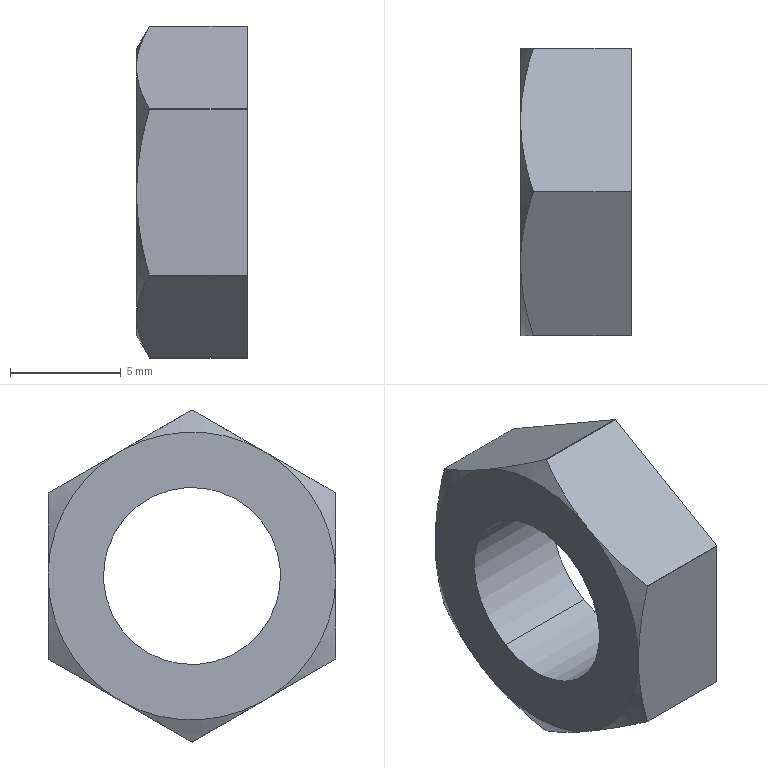Part | STEP file | SANBN8-40-Part-2-1 | 1 solid | 20 faces | box 5 x 13 x 15 mm | volume 477.717 mm3 | plane 8 | cylinder 6 | cone 6 | commonest cylinder face diameters 15 x4 8 x2
STEP:
#1=CARTESIAN_POINT('',(12.5,2.,-3.464));
#2=VERTEX_POINT('',#1);
#3=CARTESIAN_POINT('',(12.5,-2.,3.464));
#4=VERTEX_POINT('',#3);
#5=CARTESIAN_POINT('',(12.5,0.,0.));
#6=DIRECTION('',(-1.,0.,0.));
#7=DIRECTION('',(0.,-0.5,0.866));
#8=AXIS2_PLACEMENT_3D('',#5,#6,#7);
#9=CIRCLE('',#8,4.);
#10=EDGE_CURVE('',#2,#4,#9,.T.);
#11=ORIENTED_EDGE('',*,*,#10,.T.);
#12=CARTESIAN_POINT('',(17.5,-2.,3.464));
#13=VERTEX_POINT('',#12);
#14=CARTESIAN_POINT('',(42.5,-2.,3.464));
#15=DIRECTION('',(1.,0.,0.));
#16=VECTOR('',#15,1000.);
#17=LINE('',#14,#16);
#18=EDGE_CURVE('',#4,#13,#17,.T.);
#19=ORIENTED_EDGE('',*,*,#18,.T.);
#20=CARTESIAN_POINT('',(17.5,2.,-3.464));
#21=VERTEX_POINT('',#20);
#22=CARTESIAN_POINT('',(17.5,0.,0.));
#23=DIRECTION('',(1.,0.,0.));
#24=DIRECTION('',(0.,0.5,-0.866));
#25=AXIS2_PLACEMENT_3D('',#22,#23,#24);
#26=CIRCLE('',#25,4.);
#27=EDGE_CURVE('',#13,#21,#26,.T.);
#28=ORIENTED_EDGE('',*,*,#27,.T.);
#29=CARTESIAN_POINT('',(42.5,2.,-3.464));
#30=DIRECTION('',(1.,0.,0.));
#31=VECTOR('',#30,1000.);
#32=LINE('',#29,#31);
#33=EDGE_CURVE('',#2,#21,#32,.T.);
#34=ORIENTED_EDGE('',*,*,#33,.F.);
#35=EDGE_LOOP('',(#11,#19,#28,#34));
#36=FACE_OUTER_BOUND('',#35,.T.);
#37=CARTESIAN_POINT('',(42.5,0.,0.));
#38=DIRECTION('',(1.,0.,0.));
#39=DIRECTION('',(0.,0.5,-0.866));
#40=AXIS2_PLACEMENT_3D('',#37,#38,#39);
#41=CYLINDRICAL_SURFACE('',#40,4.);
#42=ADVANCED_FACE('',(#36),#41,.F.);
#43=CARTESIAN_POINT('',(17.5,0.009615,7.5));
#44=VERTEX_POINT('',#43);
#45=CARTESIAN_POINT('',(17.5,-0.00963,7.5));
#46=VERTEX_POINT('',#45);
#47=CARTESIAN_POINT('',(17.5,0.,0.));
#48=DIRECTION('',(1.,0.,0.));
#49=DIRECTION('',(0.,0.5,-0.866));
#50=AXIS2_PLACEMENT_3D('',#47,#48,#49);
#51=CIRCLE('',#50,7.5);
#52=EDGE_CURVE('',#44,#46,#51,.T.);
#53=ORIENTED_EDGE('',*,*,#52,.F.);
#54=CARTESIAN_POINT('',(13.077,0.009615,7.5));
#55=VERTEX_POINT('',#54);
#56=CARTESIAN_POINT('',(12.5,0.009615,7.5));
#57=DIRECTION('',(1.,0.,0.));
#58=VECTOR('',#57,1000.);
#59=LINE('',#56,#58);
#60=EDGE_CURVE('',#55,#44,#59,.T.);
#61=ORIENTED_EDGE('',*,*,#60,.F.);
#62=CARTESIAN_POINT('',(13.077,-0.00963,7.5));
#63=VERTEX_POINT('',#62);
#64=CARTESIAN_POINT('',(13.077,0.,0.));
#65=DIRECTION('',(1.,0.,0.));
#66=DIRECTION('',(0.,0.5,-0.866));
#67=AXIS2_PLACEMENT_3D('',#64,#65,#66);
#68=CIRCLE('',#67,7.5);
#69=EDGE_CURVE('',#55,#63,#68,.T.);
#70=ORIENTED_EDGE('',*,*,#69,.T.);
#71=CARTESIAN_POINT('',(12.5,-0.00963,7.5));
#72=DIRECTION('',(-1.,0.,0.));
#73=VECTOR('',#72,1000.);
#74=LINE('',#71,#73);
#75=EDGE_CURVE('',#46,#63,#74,.T.);
#76=ORIENTED_EDGE('',*,*,#75,.F.);
#77=EDGE_LOOP('',(#53,#61,#70,#76));
#78=FACE_OUTER_BOUND('',#77,.T.);
#79=CARTESIAN_POINT('',(12.5,0.,0.));
#80=DIRECTION('',(-1.,0.,0.));
#81=DIRECTION('',(0.,0.5,-0.866));
#82=AXIS2_PLACEMENT_3D('',#79,#80,#81);
#83=CYLINDRICAL_SURFACE('',#82,7.5);
#84=ADVANCED_FACE('',(#78),#83,.T.);
#85=CARTESIAN_POINT('',(17.5,-0.009615,-7.5));
#86=VERTEX_POINT('',#85);
#87=CARTESIAN_POINT('',(17.5,0.00963,-7.5));
#88=VERTEX_POINT('',#87);
#89=CARTESIAN_POINT('',(17.5,0.,0.));
#90=DIRECTION('',(1.,0.,0.));
#91=DIRECTION('',(0.,0.5,-0.866));
#92=AXIS2_PLACEMENT_3D('',#89,#90,#91);
#93=CIRCLE('',#92,7.5);
#94=EDGE_CURVE('',#86,#88,#93,.T.);
#95=ORIENTED_EDGE('',*,*,#94,.F.);
#96=CARTESIAN_POINT('',(13.077,-0.009615,-7.5));
#97=VERTEX_POINT('',#96);
#98=CARTESIAN_POINT('',(12.5,-0.009615,-7.5));
#99=DIRECTION('',(1.,0.,0.));
#100=VECTOR('',#99,1000.);
#101=LINE('',#98,#100);
#102=EDGE_CURVE('',#97,#86,#101,.T.);
#103=ORIENTED_EDGE('',*,*,#102,.F.);
#104=CARTESIAN_POINT('',(13.077,0.00963,-7.5));
#105=VERTEX_POINT('',#104);
#106=CARTESIAN_POINT('',(13.077,0.,0.));
#107=DIRECTION('',(1.,0.,0.));
#108=DIRECTION('',(0.,0.5,-0.866));
#109=AXIS2_PLACEMENT_3D('',#106,#107,#108);
#110=CIRCLE('',#109,7.5);
#111=EDGE_CURVE('',#97,#105,#110,.T.);
#112=ORIENTED_EDGE('',*,*,#111,.T.);
#113=CARTESIAN_POINT('',(12.5,0.00963,-7.5));
#114=DIRECTION('',(-1.,0.,0.));
#115=VECTOR('',#114,1000.);
#116=LINE('',#113,#115);
#117=EDGE_CURVE('',#88,#105,#116,.T.);
#118=ORIENTED_EDGE('',*,*,#117,.F.);
#119=EDGE_LOOP('',(#95,#103,#112,#118));
#120=FACE_OUTER_BOUND('',#119,.T.);
#121=CARTESIAN_POINT('',(12.5,0.,0.));
#122=DIRECTION('',(-1.,0.,0.));
#123=DIRECTION('',(0.,0.5,-0.866));
#124=AXIS2_PLACEMENT_3D('',#121,#122,#123);
#125=CYLINDRICAL_SURFACE('',#124,7.5);
#126=ADVANCED_FACE('',(#120),#125,.T.);
#127=CARTESIAN_POINT('',(13.077,-6.49,3.758));
#128=VERTEX_POINT('',#127);
#129=CARTESIAN_POINT('',(13.077,-6.5,3.742));
#130=VERTEX_POINT('',#129);
#131=CARTESIAN_POINT('',(13.077,0.,0.));
#132=DIRECTION('',(1.,0.,0.));
#133=DIRECTION('',(0.,0.5,-0.866));
#134=AXIS2_PLACEMENT_3D('',#131,#132,#133);
#135=CIRCLE('',#134,7.5);
#136=EDGE_CURVE('',#128,#130,#135,.T.);
#137=ORIENTED_EDGE('',*,*,#136,.T.);
#138=CARTESIAN_POINT('',(17.5,-6.5,3.742));
#139=VERTEX_POINT('',#138);
#140=CARTESIAN_POINT('',(12.5,-6.5,3.742));
#141=DIRECTION('',(-1.,0.,0.));
#142=VECTOR('',#141,1000.);
#143=LINE('',#140,#142);
#144=EDGE_CURVE('',#139,#130,#143,.T.);
#145=ORIENTED_EDGE('',*,*,#144,.F.);
#146=CARTESIAN_POINT('',(17.5,-6.49,3.758));
#147=VERTEX_POINT('',#146);
#148=CARTESIAN_POINT('',(17.5,0.,0.));
#149=DIRECTION('',(1.,0.,0.));
#150=DIRECTION('',(0.,0.5,-0.866));
#151=AXIS2_PLACEMENT_3D('',#148,#149,#150);
#152=CIRCLE('',#151,7.5);
#153=EDGE_CURVE('',#147,#139,#152,.T.);
#154=ORIENTED_EDGE('',*,*,#153,.F.);
#155=CARTESIAN_POINT('',(12.5,-6.49,3.758));
#156=DIRECTION('',(1.,0.,0.));
#157=VECTOR('',#156,1000.);
#158=LINE('',#155,#157);
#159=EDGE_CURVE('',#128,#147,#158,.T.);
#160=ORIENTED_EDGE('',*,*,#159,.F.);
#161=EDGE_LOOP('',(#137,#145,#154,#160));
#162=FACE_OUTER_BOUND('',#161,.T.);
#163=CARTESIAN_POINT('',(12.5,0.,0.));
#164=DIRECTION('',(-1.,0.,0.));
#165=DIRECTION('',(0.,0.5,-0.866));
#166=AXIS2_PLACEMENT_3D('',#163,#164,#165);
#167=CYLINDRICAL_SURFACE('',#166,7.5);
#168=ADVANCED_FACE('',(#162),#167,.T.);
#169=ORIENTED_EDGE('',*,*,#69,.F.);
#170=CARTESIAN_POINT('',(12.5,3.099,5.714));
#171=VERTEX_POINT('',#170);
#172=CARTESIAN_POINT('',(12.5,3.099,5.714));
#173=CARTESIAN_POINT('',(12.51,2.573,6.018));
#174=CARTESIAN_POINT('',(12.569,2.052,6.319));
#175=CARTESIAN_POINT('',(12.769,1.023,6.914));
#176=CARTESIAN_POINT('',(12.909,0.5143,7.208));
#177=CARTESIAN_POINT('',(13.077,0.009615,7.5));
#178=B_SPLINE_CURVE_WITH_KNOTS('',3,(#172,#173,#174,#175,#176,#177),.UNSPECIFIED.,.F.,.F.,(4,2,4),(0.003966,0.005766,0.007567),.UNSPECIFIED.);
#179=EDGE_CURVE('',#171,#55,#178,.T.);
#180=ORIENTED_EDGE('',*,*,#179,.F.);
#181=CARTESIAN_POINT('',(12.5,-3.25,5.629));
#182=VERTEX_POINT('',#181);
#183=CARTESIAN_POINT('',(12.5,0.,0.));
#184=DIRECTION('',(1.,0.,0.));
#185=DIRECTION('',(0.,0.5,-0.866));
#186=AXIS2_PLACEMENT_3D('',#183,#184,#185);
#187=CIRCLE('',#186,6.5);
#188=EDGE_CURVE('',#171,#182,#187,.T.);
#189=ORIENTED_EDGE('',*,*,#188,.T.);
#190=CARTESIAN_POINT('',(13.077,-0.00963,7.5));
#191=CARTESIAN_POINT('',(12.726,-1.065,6.89));
#192=CARTESIAN_POINT('',(12.5,-2.14,6.27));
#193=CARTESIAN_POINT('',(12.5,-3.25,5.629));
#194=B_SPLINE_CURVE_WITH_KNOTS('',3,(#190,#191,#192,#193),.UNSPECIFIED.,.F.,.F.,(4,4),(0.008188,0.01199),.UNSPECIFIED.);
#195=EDGE_CURVE('',#63,#182,#194,.T.);
#196=ORIENTED_EDGE('',*,*,#195,.F.);
#197=EDGE_LOOP('',(#169,#180,#189,#196));
#198=FACE_OUTER_BOUND('',#197,.T.);
#199=CARTESIAN_POINT('',(13.077,0.,0.));
#200=DIRECTION('',(1.,0.,0.));
#201=DIRECTION('',(0.,-0.5,0.866));
#202=AXIS2_PLACEMENT_3D('',#199,#200,#201);
#203=CONICAL_SURFACE('',#202,7.5,1.047);
#204=ADVANCED_FACE('',(#198),#203,.T.);
#205=CARTESIAN_POINT('',(12.5,-6.498,0.1727));
#206=VERTEX_POINT('',#205);
#207=CARTESIAN_POINT('',(12.5,0.,0.));
#208=DIRECTION('',(1.,0.,0.));
#209=DIRECTION('',(0.,0.5,-0.866));
#210=AXIS2_PLACEMENT_3D('',#207,#208,#209);
#211=CIRCLE('',#210,6.5);
#212=EDGE_CURVE('',#182,#206,#211,.T.);
#213=ORIENTED_EDGE('',*,*,#212,.T.);
#214=CARTESIAN_POINT('',(13.077,-6.5,3.742));
#215=CARTESIAN_POINT('',(12.74,-6.499,2.573));
#216=CARTESIAN_POINT('',(12.519,-6.498,1.387));
#217=CARTESIAN_POINT('',(12.5,-6.498,0.1727));
#218=B_SPLINE_CURVE_WITH_KNOTS('',3,(#214,#215,#216,#217),.UNSPECIFIED.,.F.,.F.,(4,4),(0.000002502,0.003617),.UNSPECIFIED.);
#219=EDGE_CURVE('',#130,#206,#218,.T.);
#220=ORIENTED_EDGE('',*,*,#219,.F.);
#221=ORIENTED_EDGE('',*,*,#136,.F.);
#222=CARTESIAN_POINT('',(12.5,-3.25,5.629));
#223=CARTESIAN_POINT('',(12.5,-3.805,5.309));
#224=CARTESIAN_POINT('',(12.556,-4.352,4.993));
#225=CARTESIAN_POINT('',(12.757,-5.431,4.37));
#226=CARTESIAN_POINT('',(12.902,-5.963,4.063));
#227=CARTESIAN_POINT('',(13.077,-6.49,3.758));
#228=B_SPLINE_CURVE_WITH_KNOTS('',3,(#222,#223,#224,#225,#226,#227),.UNSPECIFIED.,.F.,.F.,(4,2,4),(0.01199,0.0139,0.0158),.UNSPECIFIED.);
#229=EDGE_CURVE('',#182,#128,#228,.T.);
#230=ORIENTED_EDGE('',*,*,#229,.F.);
#231=EDGE_LOOP('',(#213,#220,#221,#230));
#232=FACE_OUTER_BOUND('',#231,.T.);
#233=CARTESIAN_POINT('',(13.077,0.,0.));
#234=DIRECTION('',(1.,0.,0.));
#235=DIRECTION('',(0.,-0.5,0.866));
#236=AXIS2_PLACEMENT_3D('',#233,#234,#235);
#237=CONICAL_SURFACE('',#236,7.5,1.047);
#238=ADVANCED_FACE('',(#232),#237,.T.);
#239=CARTESIAN_POINT('',(13.077,6.49,-3.758));
#240=VERTEX_POINT('',#239);
#241=CARTESIAN_POINT('',(13.077,6.5,-3.742));
#242=VERTEX_POINT('',#241);
#243=CARTESIAN_POINT('',(13.077,0.,0.));
#244=DIRECTION('',(1.,0.,0.));
#245=DIRECTION('',(0.,0.5,-0.866));
#246=AXIS2_PLACEMENT_3D('',#243,#244,#245);
#247=CIRCLE('',#246,7.5);
#248=EDGE_CURVE('',#240,#242,#247,.T.);
#249=ORIENTED_EDGE('',*,*,#248,.F.);
#250=CARTESIAN_POINT('',(12.5,3.25,-5.629));
#251=VERTEX_POINT('',#250);
#252=CARTESIAN_POINT('',(12.5,3.25,-5.629));
#253=CARTESIAN_POINT('',(12.5,3.805,-5.309));
#254=CARTESIAN_POINT('',(12.556,4.352,-4.993));
#255=CARTESIAN_POINT('',(12.757,5.431,-4.37));
#256=CARTESIAN_POINT('',(12.902,5.963,-4.063));
#257=CARTESIAN_POINT('',(13.077,6.49,-3.758));
#258=B_SPLINE_CURVE_WITH_KNOTS('',3,(#252,#253,#254,#255,#256,#257),.UNSPECIFIED.,.F.,.F.,(4,2,4),(0.01199,0.0139,0.0158),.UNSPECIFIED.);
#259=EDGE_CURVE('',#251,#240,#258,.T.);
#260=ORIENTED_EDGE('',*,*,#259,.F.);
#261=CARTESIAN_POINT('',(12.5,6.498,-0.1727));
#262=VERTEX_POINT('',#261);
#263=CARTESIAN_POINT('',(12.5,0.,0.));
#264=DIRECTION('',(1.,0.,0.));
#265=DIRECTION('',(0.,0.5,-0.866));
#266=AXIS2_PLACEMENT_3D('',#263,#264,#265);
#267=CIRCLE('',#266,6.5);
#268=EDGE_CURVE('',#251,#262,#267,.T.);
#269=ORIENTED_EDGE('',*,*,#268,.T.);
#270=CARTESIAN_POINT('',(13.077,6.5,-3.742));
#271=CARTESIAN_POINT('',(12.74,6.499,-2.573));
#272=CARTESIAN_POINT('',(12.519,6.498,-1.387));
#273=CARTESIAN_POINT('',(12.5,6.498,-0.1727));
#274=B_SPLINE_CURVE_WITH_KNOTS('',3,(#270,#271,#272,#273),.UNSPECIFIED.,.F.,.F.,(4,4),(0.000002502,0.003617),.UNSPECIFIED.);
#275=EDGE_CURVE('',#242,#262,#274,.T.);
#276=ORIENTED_EDGE('',*,*,#275,.F.);
#277=EDGE_LOOP('',(#249,#260,#269,#276));
#278=FACE_OUTER_BOUND('',#277,.T.);
#279=CARTESIAN_POINT('',(13.077,0.,0.));
#280=DIRECTION('',(1.,0.,0.));
#281=DIRECTION('',(0.,-0.5,0.866));
#282=AXIS2_PLACEMENT_3D('',#279,#280,#281);
#283=CONICAL_SURFACE('',#282,7.5,1.047);
#284=ADVANCED_FACE('',(#278),#283,.T.);
#285=ORIENTED_EDGE('',*,*,#111,.F.);
#286=CARTESIAN_POINT('',(12.5,-3.099,-5.714));
#287=VERTEX_POINT('',#286);
#288=CARTESIAN_POINT('',(12.5,-3.099,-5.714));
#289=CARTESIAN_POINT('',(12.51,-2.573,-6.018));
#290=CARTESIAN_POINT('',(12.569,-2.052,-6.319));
#291=CARTESIAN_POINT('',(12.769,-1.023,-6.914));
#292=CARTESIAN_POINT('',(12.909,-0.5143,-7.208));
#293=CARTESIAN_POINT('',(13.077,-0.009615,-7.5));
#294=B_SPLINE_CURVE_WITH_KNOTS('',3,(#288,#289,#290,#291,#292,#293),.UNSPECIFIED.,.F.,.F.,(4,2,4),(0.003966,0.005766,0.007567),.UNSPECIFIED.);
#295=EDGE_CURVE('',#287,#97,#294,.T.);
#296=ORIENTED_EDGE('',*,*,#295,.F.);
#297=CARTESIAN_POINT('',(12.5,0.,0.));
#298=DIRECTION('',(1.,0.,0.));
#299=DIRECTION('',(0.,0.5,-0.866));
#300=AXIS2_PLACEMENT_3D('',#297,#298,#299);
#301=CIRCLE('',#300,6.5);
#302=EDGE_CURVE('',#287,#251,#301,.T.);
#303=ORIENTED_EDGE('',*,*,#302,.T.);
#304=CARTESIAN_POINT('',(13.077,0.00963,-7.5));
#305=CARTESIAN_POINT('',(12.726,1.065,-6.89));
#306=CARTESIAN_POINT('',(12.5,2.14,-6.27));
#307=CARTESIAN_POINT('',(12.5,3.25,-5.629));
#308=B_SPLINE_CURVE_WITH_KNOTS('',3,(#304,#305,#306,#307),.UNSPECIFIED.,.F.,.F.,(4,4),(0.008188,0.01199),.UNSPECIFIED.);
#309=EDGE_CURVE('',#105,#251,#308,.T.);
#310=ORIENTED_EDGE('',*,*,#309,.F.);
#311=EDGE_LOOP('',(#285,#296,#303,#310));
#312=FACE_OUTER_BOUND('',#311,.T.);
#313=CARTESIAN_POINT('',(13.077,0.,0.));
#314=DIRECTION('',(1.,0.,0.));
#315=DIRECTION('',(0.,-0.5,0.866));
#316=AXIS2_PLACEMENT_3D('',#313,#314,#315);
#317=CONICAL_SURFACE('',#316,7.5,1.047);
#318=ADVANCED_FACE('',(#312),#317,.T.);
#319=CARTESIAN_POINT('',(12.5,6.497,0.181));
#320=VERTEX_POINT('',#319);
#321=CARTESIAN_POINT('',(12.5,3.406,5.536));
#322=VERTEX_POINT('',#321);
#323=CARTESIAN_POINT('',(12.5,0.,0.));
#324=DIRECTION('',(1.,0.,0.));
#325=DIRECTION('',(0.,0.5,-0.866));
#326=AXIS2_PLACEMENT_3D('',#323,#324,#325);
#327=CIRCLE('',#326,6.5);
#328=EDGE_CURVE('',#320,#322,#327,.T.);
#329=ORIENTED_EDGE('',*,*,#328,.T.);
#330=CARTESIAN_POINT('',(13.077,6.495,3.75));
#331=VERTEX_POINT('',#330);
#332=CARTESIAN_POINT('',(13.077,6.495,3.75));
#333=CARTESIAN_POINT('',(12.74,5.483,4.335));
#334=CARTESIAN_POINT('',(12.519,4.457,4.929));
#335=CARTESIAN_POINT('',(12.5,3.406,5.536));
#336=B_SPLINE_CURVE_WITH_KNOTS('',3,(#332,#333,#334,#335),.UNSPECIFIED.,.F.,.F.,(4,4),(0.000000833,0.003616),.UNSPECIFIED.);
#337=EDGE_CURVE('',#331,#322,#336,.T.);
#338=ORIENTED_EDGE('',*,*,#337,.F.);
#339=CARTESIAN_POINT('',(12.5,6.497,0.181));
#340=CARTESIAN_POINT('',(12.51,6.497,0.7887));
#341=CARTESIAN_POINT('',(12.569,6.497,1.391));
#342=CARTESIAN_POINT('',(12.769,6.496,2.579));
#343=CARTESIAN_POINT('',(12.909,6.496,3.167));
#344=CARTESIAN_POINT('',(13.077,6.495,3.75));
#345=B_SPLINE_CURVE_WITH_KNOTS('',3,(#339,#340,#341,#342,#343,#344),.UNSPECIFIED.,.F.,.F.,(4,2,4),(0.003967,0.005768,0.007568),.UNSPECIFIED.);
#346=EDGE_CURVE('',#320,#331,#345,.T.);
#347=ORIENTED_EDGE('',*,*,#346,.F.);
#348=EDGE_LOOP('',(#329,#338,#347));
#349=FACE_OUTER_BOUND('',#348,.T.);
#350=CARTESIAN_POINT('',(13.077,0.,0.));
#351=DIRECTION('',(1.,0.,0.));
#352=DIRECTION('',(0.,-0.5,0.866));
#353=AXIS2_PLACEMENT_3D('',#350,#351,#352);
#354=CONICAL_SURFACE('',#353,7.5,1.047);
#355=ADVANCED_FACE('',(#349),#354,.T.);
#356=CARTESIAN_POINT('',(17.5,6.495,3.75));
#357=VERTEX_POINT('',#356);
#358=CARTESIAN_POINT('',(17.5,6.495,3.75));
#359=DIRECTION('',(0.,-0.8657,0.5006));
#360=VECTOR('',#359,1000.);
#361=LINE('',#358,#360);
#362=EDGE_CURVE('',#357,#44,#361,.T.);
#363=ORIENTED_EDGE('',*,*,#362,.T.);
#364=ORIENTED_EDGE('',*,*,#52,.T.);
#365=CARTESIAN_POINT('',(17.5,0.,7.506));
#366=DIRECTION('',(0.,-0.866,-0.5));
#367=VECTOR('',#366,1000.);
#368=LINE('',#365,#367);
#369=EDGE_CURVE('',#46,#147,#368,.T.);
#370=ORIENTED_EDGE('',*,*,#369,.T.);
#371=ORIENTED_EDGE('',*,*,#153,.T.);
#372=CARTESIAN_POINT('',(17.5,-6.495,-3.75));
#373=VERTEX_POINT('',#372);
#374=CARTESIAN_POINT('',(17.5,-6.5,3.753));
#375=DIRECTION('',(0.,0.000641,-1.));
#376=VECTOR('',#375,1000.);
#377=LINE('',#374,#376);
#378=EDGE_CURVE('',#139,#373,#377,.T.);
#379=ORIENTED_EDGE('',*,*,#378,.T.);
#380=CARTESIAN_POINT('',(17.5,-6.495,-3.75));
#381=DIRECTION('',(0.,0.8657,-0.5006));
#382=VECTOR('',#381,1000.);
#383=LINE('',#380,#382);
#384=EDGE_CURVE('',#373,#86,#383,.T.);
#385=ORIENTED_EDGE('',*,*,#384,.T.);
#386=ORIENTED_EDGE('',*,*,#94,.T.);
#387=CARTESIAN_POINT('',(17.5,6.49,-3.758));
#388=VERTEX_POINT('',#387);
#389=CARTESIAN_POINT('',(17.5,0.,-7.506));
#390=DIRECTION('',(0.,0.866,0.5));
#391=VECTOR('',#390,1000.);
#392=LINE('',#389,#391);
#393=EDGE_CURVE('',#88,#388,#392,.T.);
#394=ORIENTED_EDGE('',*,*,#393,.T.);
#395=CARTESIAN_POINT('',(17.5,6.5,-3.742));
#396=VERTEX_POINT('',#395);
#397=CARTESIAN_POINT('',(17.5,0.,0.));
#398=DIRECTION('',(1.,0.,0.));
#399=DIRECTION('',(0.,0.5,-0.866));
#400=AXIS2_PLACEMENT_3D('',#397,#398,#399);
#401=CIRCLE('',#400,7.5);
#402=EDGE_CURVE('',#388,#396,#401,.T.);
#403=ORIENTED_EDGE('',*,*,#402,.T.);
#404=CARTESIAN_POINT('',(17.5,6.5,-3.753));
#405=DIRECTION('',(0.,-0.000641,1.));
#406=VECTOR('',#405,1000.);
#407=LINE('',#404,#406);
#408=EDGE_CURVE('',#396,#357,#407,.T.);
#409=ORIENTED_EDGE('',*,*,#408,.T.);
#410=EDGE_LOOP('',(#363,#364,#370,#371,#379,#385,#386,#394,#403,#409));
#411=FACE_OUTER_BOUND('',#410,.T.);
#412=CARTESIAN_POINT('',(17.5,0.,0.));
#413=DIRECTION('',(1.,0.,0.));
#414=DIRECTION('',(0.,0.5,-0.866));
#415=AXIS2_PLACEMENT_3D('',#412,#413,#414);
#416=CIRCLE('',#415,4.);
#417=EDGE_CURVE('',#21,#13,#416,.T.);
#418=ORIENTED_EDGE('',*,*,#417,.F.);
#419=ORIENTED_EDGE('',*,*,#27,.F.);
#420=EDGE_LOOP('',(#418,#419));
#421=FACE_BOUND('',#420,.T.);
#422=CARTESIAN_POINT('',(17.5,0.,0.));
#423=DIRECTION('',(-1.,0.,0.));
#424=DIRECTION('',(0.,0.5,-0.866));
#425=AXIS2_PLACEMENT_3D('',#422,#423,#424);
#426=PLANE('',#425);
#427=ADVANCED_FACE('',(#411,#421),#426,.F.);
#428=ORIENTED_EDGE('',*,*,#402,.F.);
#429=CARTESIAN_POINT('',(12.5,6.49,-3.758));
#430=DIRECTION('',(1.,0.,0.));
#431=VECTOR('',#430,1000.);
#432=LINE('',#429,#431);
#433=EDGE_CURVE('',#240,#388,#432,.T.);
#434=ORIENTED_EDGE('',*,*,#433,.F.);
#435=ORIENTED_EDGE('',*,*,#248,.T.);
#436=CARTESIAN_POINT('',(12.5,6.5,-3.742));
#437=DIRECTION('',(-1.,0.,0.));
#438=VECTOR('',#437,1000.);
#439=LINE('',#436,#438);
#440=EDGE_CURVE('',#396,#242,#439,.T.);
#441=ORIENTED_EDGE('',*,*,#440,.F.);
#442=EDGE_LOOP('',(#428,#434,#435,#441));
#443=FACE_OUTER_BOUND('',#442,.T.);
#444=CARTESIAN_POINT('',(12.5,0.,0.));
#445=DIRECTION('',(-1.,0.,0.));
#446=DIRECTION('',(0.,0.5,-0.866));
#447=AXIS2_PLACEMENT_3D('',#444,#445,#446);
#448=CYLINDRICAL_SURFACE('',#447,7.5);
#449=ADVANCED_FACE('',(#443),#448,.T.);
#450=CARTESIAN_POINT('',(12.5,-6.497,-0.181));
#451=VERTEX_POINT('',#450);
#452=CARTESIAN_POINT('',(13.077,-6.495,-3.75));
#453=VERTEX_POINT('',#452);
#454=CARTESIAN_POINT('',(12.5,-6.497,-0.181));
#455=CARTESIAN_POINT('',(12.51,-6.497,-0.7887));
#456=CARTESIAN_POINT('',(12.569,-6.497,-1.391));
#457=CARTESIAN_POINT('',(12.769,-6.496,-2.579));
#458=CARTESIAN_POINT('',(12.909,-6.496,-3.167));
#459=CARTESIAN_POINT('',(13.077,-6.495,-3.75));
#460=B_SPLINE_CURVE_WITH_KNOTS('',3,(#454,#455,#456,#457,#458,#459),.UNSPECIFIED.,.F.,.F.,(4,2,4),(0.003967,0.005768,0.007568),.UNSPECIFIED.);
#461=EDGE_CURVE('',#451,#453,#460,.T.);
#462=ORIENTED_EDGE('',*,*,#461,.F.);
#463=CARTESIAN_POINT('',(12.5,-3.406,-5.536));
#464=VERTEX_POINT('',#463);
#465=CARTESIAN_POINT('',(12.5,0.,0.));
#466=DIRECTION('',(1.,0.,0.));
#467=DIRECTION('',(0.,0.5,-0.866));
#468=AXIS2_PLACEMENT_3D('',#465,#466,#467);
#469=CIRCLE('',#468,6.5);
#470=EDGE_CURVE('',#451,#464,#469,.T.);
#471=ORIENTED_EDGE('',*,*,#470,.T.);
#472=CARTESIAN_POINT('',(13.077,-6.495,-3.75));
#473=CARTESIAN_POINT('',(12.74,-5.483,-4.335));
#474=CARTESIAN_POINT('',(12.519,-4.457,-4.929));
#475=CARTESIAN_POINT('',(12.5,-3.406,-5.536));
#476=B_SPLINE_CURVE_WITH_KNOTS('',3,(#472,#473,#474,#475),.UNSPECIFIED.,.F.,.F.,(4,4),(0.000000833,0.003616),.UNSPECIFIED.);
#477=EDGE_CURVE('',#453,#464,#476,.T.);
#478=ORIENTED_EDGE('',*,*,#477,.F.);
#479=EDGE_LOOP('',(#462,#471,#478));
#480=FACE_OUTER_BOUND('',#479,.T.);
#481=CARTESIAN_POINT('',(13.077,0.,0.));
#482=DIRECTION('',(1.,0.,0.));
#483=DIRECTION('',(0.,-0.5,0.866));
#484=AXIS2_PLACEMENT_3D('',#481,#482,#483);
#485=CONICAL_SURFACE('',#484,7.5,1.047);
#486=ADVANCED_FACE('',(#480),#485,.T.);
#487=ORIENTED_EDGE('',*,*,#10,.F.);
#488=CARTESIAN_POINT('',(12.5,0.,0.));
#489=DIRECTION('',(-1.,0.,0.));
#490=DIRECTION('',(0.,-0.5,0.866));
#491=AXIS2_PLACEMENT_3D('',#488,#489,#490);
#492=CIRCLE('',#491,4.);
#493=EDGE_CURVE('',#4,#2,#492,.T.);
#494=ORIENTED_EDGE('',*,*,#493,.F.);
#495=EDGE_LOOP('',(#487,#494));
#496=FACE_BOUND('',#495,.T.);
#497=CARTESIAN_POINT('',(12.5,6.498,-0.1727));
#498=DIRECTION('',(0.,-0.000641,1.));
#499=VECTOR('',#498,1000.);
#500=LINE('',#497,#499);
#501=EDGE_CURVE('',#262,#320,#500,.T.);
#502=ORIENTED_EDGE('',*,*,#501,.F.);
#503=ORIENTED_EDGE('',*,*,#268,.F.);
#504=ORIENTED_EDGE('',*,*,#302,.F.);
#505=CARTESIAN_POINT('',(12.5,-3.406,-5.536));
#506=DIRECTION('',(0.,0.8657,-0.5006));
#507=VECTOR('',#506,1000.);
#508=LINE('',#505,#507);
#509=EDGE_CURVE('',#464,#287,#508,.T.);
#510=ORIENTED_EDGE('',*,*,#509,.F.);
#511=ORIENTED_EDGE('',*,*,#470,.F.);
#512=CARTESIAN_POINT('',(12.5,-6.498,0.1727));
#513=DIRECTION('',(0.,0.000641,-1.));
#514=VECTOR('',#513,1000.);
#515=LINE('',#512,#514);
#516=EDGE_CURVE('',#206,#451,#515,.T.);
#517=ORIENTED_EDGE('',*,*,#516,.F.);
#518=ORIENTED_EDGE('',*,*,#212,.F.);
#519=ORIENTED_EDGE('',*,*,#188,.F.);
#520=CARTESIAN_POINT('',(12.5,3.406,5.536));
#521=DIRECTION('',(0.,-0.8657,0.5006));
#522=VECTOR('',#521,1000.);
#523=LINE('',#520,#522);
#524=EDGE_CURVE('',#322,#171,#523,.T.);
#525=ORIENTED_EDGE('',*,*,#524,.F.);
#526=ORIENTED_EDGE('',*,*,#328,.F.);
#527=EDGE_LOOP('',(#502,#503,#504,#510,#511,#517,#518,#519,#525,#526));
#528=FACE_OUTER_BOUND('',#527,.T.);
#529=CARTESIAN_POINT('',(12.5,5.629,3.25));
#530=DIRECTION('',(1.,0.,0.));
#531=DIRECTION('',(0.,-0.5,0.866));
#532=AXIS2_PLACEMENT_3D('',#529,#530,#531);
#533=PLANE('',#532);
#534=ADVANCED_FACE('',(#496,#528),#533,.F.);
#535=CARTESIAN_POINT('',(12.5,-6.495,-3.75));
#536=DIRECTION('',(1.,0.,0.));
#537=VECTOR('',#536,1000.);
#538=LINE('',#535,#537);
#539=EDGE_CURVE('',#453,#373,#538,.T.);
#540=ORIENTED_EDGE('',*,*,#539,.F.);
#541=ORIENTED_EDGE('',*,*,#477,.T.);
#542=ORIENTED_EDGE('',*,*,#509,.T.);
#543=ORIENTED_EDGE('',*,*,#295,.T.);
#544=ORIENTED_EDGE('',*,*,#102,.T.);
#545=ORIENTED_EDGE('',*,*,#384,.F.);
#546=EDGE_LOOP('',(#540,#541,#542,#543,#544,#545));
#547=FACE_OUTER_BOUND('',#546,.T.);
#548=CARTESIAN_POINT('',(12.5,-6.495,-3.75));
#549=DIRECTION('',(0.,0.5006,0.8657));
#550=DIRECTION('',(0.,-0.8657,0.5006));
#551=AXIS2_PLACEMENT_3D('',#548,#549,#550);
#552=PLANE('',#551);
#553=ADVANCED_FACE('',(#547),#552,.F.);
#554=ORIENTED_EDGE('',*,*,#378,.F.);
#555=ORIENTED_EDGE('',*,*,#144,.T.);
#556=ORIENTED_EDGE('',*,*,#219,.T.);
#557=ORIENTED_EDGE('',*,*,#516,.T.);
#558=ORIENTED_EDGE('',*,*,#461,.T.);
#559=ORIENTED_EDGE('',*,*,#539,.T.);
#560=EDGE_LOOP('',(#554,#555,#556,#557,#558,#559));
#561=FACE_OUTER_BOUND('',#560,.T.);
#562=CARTESIAN_POINT('',(12.5,-6.5,3.753));
#563=DIRECTION('',(0.,1.,0.000641));
#564=DIRECTION('',(0.,-0.000641,1.));
#565=AXIS2_PLACEMENT_3D('',#562,#563,#564);
#566=PLANE('',#565);
#567=ADVANCED_FACE('',(#561),#566,.F.);
#568=CARTESIAN_POINT('',(12.5,6.495,3.75));
#569=DIRECTION('',(1.,0.,0.));
#570=VECTOR('',#569,1000.);
#571=LINE('',#568,#570);
#572=EDGE_CURVE('',#331,#357,#571,.T.);
#573=ORIENTED_EDGE('',*,*,#572,.F.);
#574=ORIENTED_EDGE('',*,*,#337,.T.);
#575=ORIENTED_EDGE('',*,*,#524,.T.);
#576=ORIENTED_EDGE('',*,*,#179,.T.);
#577=ORIENTED_EDGE('',*,*,#60,.T.);
#578=ORIENTED_EDGE('',*,*,#362,.F.);
#579=EDGE_LOOP('',(#573,#574,#575,#576,#577,#578));
#580=FACE_OUTER_BOUND('',#579,.T.);
#581=CARTESIAN_POINT('',(12.5,6.495,3.75));
#582=DIRECTION('',(0.,-0.5006,-0.8657));
#583=DIRECTION('',(0.,0.8657,-0.5006));
#584=AXIS2_PLACEMENT_3D('',#581,#582,#583);
#585=PLANE('',#584);
#586=ADVANCED_FACE('',(#580),#585,.F.);
#587=ORIENTED_EDGE('',*,*,#408,.F.);
#588=ORIENTED_EDGE('',*,*,#440,.T.);
#589=ORIENTED_EDGE('',*,*,#275,.T.);
#590=ORIENTED_EDGE('',*,*,#501,.T.);
#591=ORIENTED_EDGE('',*,*,#346,.T.);
#592=ORIENTED_EDGE('',*,*,#572,.T.);
#593=EDGE_LOOP('',(#587,#588,#589,#590,#591,#592));
#594=FACE_OUTER_BOUND('',#593,.T.);
#595=CARTESIAN_POINT('',(12.5,6.5,-3.753));
#596=DIRECTION('',(0.,-1.,-0.000641));
#597=DIRECTION('',(0.,0.000641,-1.));
#598=AXIS2_PLACEMENT_3D('',#595,#596,#597);
#599=PLANE('',#598);
#600=ADVANCED_FACE('',(#594),#599,.F.);
#601=ORIENTED_EDGE('',*,*,#393,.F.);
#602=ORIENTED_EDGE('',*,*,#117,.T.);
#603=ORIENTED_EDGE('',*,*,#309,.T.);
#604=ORIENTED_EDGE('',*,*,#259,.T.);
#605=ORIENTED_EDGE('',*,*,#433,.T.);
#606=EDGE_LOOP('',(#601,#602,#603,#604,#605));
#607=FACE_OUTER_BOUND('',#606,.T.);
#608=CARTESIAN_POINT('',(12.5,0.,-7.506));
#609=DIRECTION('',(0.,-0.5,0.866));
#610=DIRECTION('',(-1.,0.,0.));
#611=AXIS2_PLACEMENT_3D('',#608,#609,#610);
#612=PLANE('',#611);
#613=ADVANCED_FACE('',(#607),#612,.F.);
#614=ORIENTED_EDGE('',*,*,#369,.F.);
#615=ORIENTED_EDGE('',*,*,#75,.T.);
#616=ORIENTED_EDGE('',*,*,#195,.T.);
#617=ORIENTED_EDGE('',*,*,#229,.T.);
#618=ORIENTED_EDGE('',*,*,#159,.T.);
#619=EDGE_LOOP('',(#614,#615,#616,#617,#618));
#620=FACE_OUTER_BOUND('',#619,.T.);
#621=CARTESIAN_POINT('',(12.5,0.,7.506));
#622=DIRECTION('',(0.,0.5,-0.866));
#623=DIRECTION('',(1.,0.,0.));
#624=AXIS2_PLACEMENT_3D('',#621,#622,#623);
#625=PLANE('',#624);
#626=ADVANCED_FACE('',(#620),#625,.F.);
#627=ORIENTED_EDGE('',*,*,#18,.F.);
#628=ORIENTED_EDGE('',*,*,#493,.T.);
#629=ORIENTED_EDGE('',*,*,#33,.T.);
#630=ORIENTED_EDGE('',*,*,#417,.T.);
#631=EDGE_LOOP('',(#627,#628,#629,#630));
#632=FACE_OUTER_BOUND('',#631,.T.);
#633=CARTESIAN_POINT('',(42.5,0.,0.));
#634=DIRECTION('',(1.,0.,0.));
#635=DIRECTION('',(0.,0.5,-0.866));
#636=AXIS2_PLACEMENT_3D('',#633,#634,#635);
#637=CYLINDRICAL_SURFACE('',#636,4.);
#638=ADVANCED_FACE('',(#632),#637,.F.);
#639=CLOSED_SHELL('',(#42,#84,#126,#168,#204,#238,#284,#318,#355,#427,#449,#486,#534,#553,#567,#586,#600,#613,#626,#638));
#640=MANIFOLD_SOLID_BREP('',#639);
#641=CARTESIAN_POINT('',(0.,0.,0.));
#642=DIRECTION('',(0.,0.,1.));
#643=DIRECTION('',(1.,0.,0.));
#644=AXIS2_PLACEMENT_3D('',#641,#642,#643);
#645=(LENGTH_UNIT()NAMED_UNIT(*)SI_UNIT(.MILLI.,.METRE.));
#646=UNCERTAINTY_MEASURE_WITH_UNIT(LENGTH_MEASURE(0.00001),#645,'','');
#647=(NAMED_UNIT(*)PLANE_ANGLE_UNIT()SI_UNIT($,.RADIAN.));
#648=(NAMED_UNIT(*)SI_UNIT($,.STERADIAN.)SOLID_ANGLE_UNIT());
#649=(GEOMETRIC_REPRESENTATION_CONTEXT(3)GLOBAL_UNCERTAINTY_ASSIGNED_CONTEXT((#646))GLOBAL_UNIT_ASSIGNED_CONTEXT((#645,#647,#648))REPRESENTATION_CONTEXT('',''));
#650=ADVANCED_BREP_SHAPE_REPRESENTATION('',(#640,#644),#649);